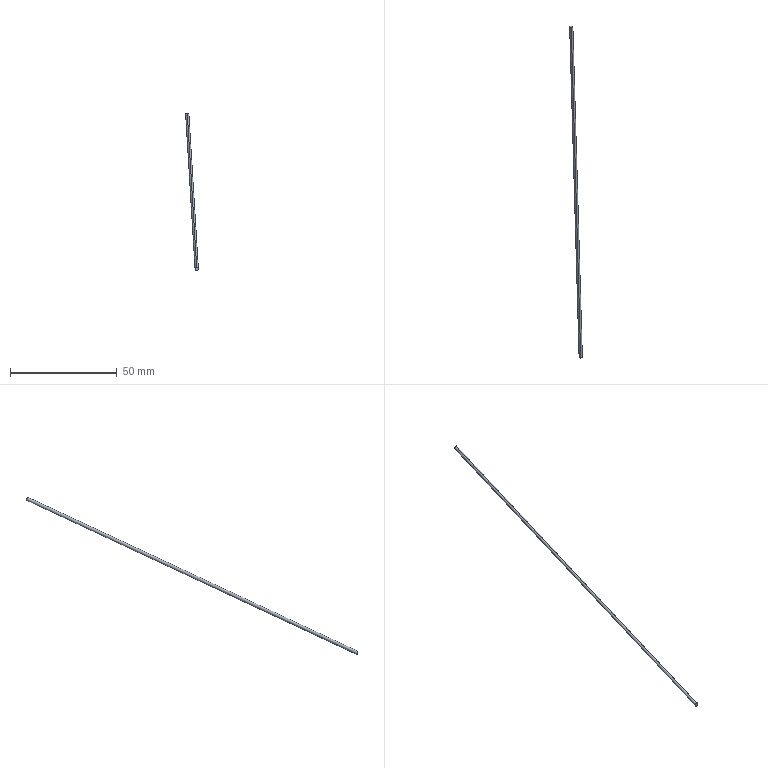Part | STEP file | 1_id790_x_t | 1 solid | 4 faces | box 5.952 x 155.177 x 73.747 mm | volume 311.788 mm3 | cylinder 2 | plane 2 | commonest cylinder face diameters 1.524 x2
STEP:
#1=CARTESIAN_POINT('',(0.,0.,0.));
#2=DIRECTION('',(0.,0.,1.));
#3=DIRECTION('',(1.,0.,0.));
#4=AXIS2_PLACEMENT_3D('',#1,#2,#3);
#5=CARTESIAN_POINT('',(978.112,154.36,-69.251));
#6=VERTEX_POINT('',#5);
#7=CARTESIAN_POINT('',(973.675,309.536,3.114));
#8=VERTEX_POINT('',#7);
#9=CARTESIAN_POINT('',(978.112,154.36,-69.251));
#10=DIRECTION('',(-0.02591,0.906,0.4225));
#11=VECTOR('',#10,1.);
#12=LINE('',#9,#11);
#13=CARTESIAN_POINT('',(976.35,215.719,-39.796));
#14=DIRECTION('',(-0.02591,0.906,0.4225));
#15=DIRECTION('',(0.002266,-0.4226,0.9063));
#16=AXIS2_PLACEMENT_3D('',#13,#14,#15);
#17=CYLINDRICAL_SURFACE('',#16,0.762);
#18=CARTESIAN_POINT('',(3.142,-68.081));
#19=DIRECTION('',(0.,1.));
#20=VECTOR('',#19,1.);
#21=LINE('',#18,#20);
#22=(GEOMETRIC_REPRESENTATION_CONTEXT(2)PARAMETRIC_REPRESENTATION_CONTEXT()REPRESENTATION_CONTEXT('',''));
#23=DEFINITIONAL_REPRESENTATION('',(#21),#22);
#24=PCURVE('',#17,#23);
#25=CARTESIAN_POINT('',(976.35,215.719,-39.796));
#26=DIRECTION('',(-0.02591,0.906,0.4225));
#27=DIRECTION('',(0.002266,-0.4226,0.9063));
#28=AXIS2_PLACEMENT_3D('',#25,#26,#27);
#29=CYLINDRICAL_SURFACE('',#28,0.762);
#30=CARTESIAN_POINT('',(3.142,-68.081));
#31=DIRECTION('',(0.,1.));
#32=VECTOR('',#31,1.);
#33=LINE('',#30,#32);
#34=(GEOMETRIC_REPRESENTATION_CONTEXT(2)PARAMETRIC_REPRESENTATION_CONTEXT()REPRESENTATION_CONTEXT('',''));
#35=DEFINITIONAL_REPRESENTATION('',(#33),#34);
#36=PCURVE('',#29,#35);
#37=SURFACE_CURVE('',#12,(#24,#36),.PCURVE_S1.);
#38=EDGE_CURVE('',#6,#8,#37,.T.);
#39=ORIENTED_EDGE('',*,*,#38,.F.);
#40=CARTESIAN_POINT('',(978.097,154.36,-67.57));
#41=VERTEX_POINT('',#40);
#42=CARTESIAN_POINT('',(978.104,154.36,-68.41));
#43=DIRECTION('',(0.,-1.,0.));
#44=DIRECTION('',(-0.0612,0.,0.9981));
#45=AXIS2_PLACEMENT_3D('',#42,#43,#44);
#46=ELLIPSE('',#45,0.8411,0.762);
#47=CARTESIAN_POINT('',(6.283,-67.37));
#48=CARTESIAN_POINT('',(6.236,-67.369));
#49=CARTESIAN_POINT('',(6.14,-67.37));
#50=CARTESIAN_POINT('',(5.998,-67.378));
#51=CARTESIAN_POINT('',(5.855,-67.393));
#52=CARTESIAN_POINT('',(5.712,-67.414));
#53=CARTESIAN_POINT('',(5.569,-67.443));
#54=CARTESIAN_POINT('',(5.426,-67.476));
#55=CARTESIAN_POINT('',(5.284,-67.515));
#56=CARTESIAN_POINT('',(5.141,-67.559));
#57=CARTESIAN_POINT('',(4.998,-67.605));
#58=CARTESIAN_POINT('',(4.855,-67.654));
#59=CARTESIAN_POINT('',(4.712,-67.705));
#60=CARTESIAN_POINT('',(4.57,-67.756));
#61=CARTESIAN_POINT('',(4.427,-67.806));
#62=CARTESIAN_POINT('',(4.284,-67.855));
#63=CARTESIAN_POINT('',(4.141,-67.901));
#64=CARTESIAN_POINT('',(3.998,-67.944));
#65=CARTESIAN_POINT('',(3.856,-67.982));
#66=CARTESIAN_POINT('',(3.713,-68.014));
#67=CARTESIAN_POINT('',(3.57,-68.041));
#68=CARTESIAN_POINT('',(3.427,-68.062));
#69=CARTESIAN_POINT('',(3.284,-68.076));
#70=CARTESIAN_POINT('',(3.189,-68.08));
#71=CARTESIAN_POINT('',(3.142,-68.081));
#72=B_SPLINE_CURVE_WITH_KNOTS('',3,(#47,#48,#49,#50,#51,#52,#53,#54,#55,#56,#57,#58,#59,#60,#61,#62,#63,#64,#65,#66,#67,#68,#69,#70,#71),.UNSPECIFIED.,.F.,.F.,(4,1,1,1,1,1,1,1,1,1,1,1,1,1,1,1,1,1,1,1,1,1,4),(6.225,6.368,6.511,6.654,6.797,6.939,7.082,7.225,7.368,7.511,7.653,7.796,7.939,8.082,8.225,8.367,8.51,8.653,8.796,8.939,9.081,9.224,9.367),.QUASI_UNIFORM_KNOTS.);
#73=(GEOMETRIC_REPRESENTATION_CONTEXT(2)PARAMETRIC_REPRESENTATION_CONTEXT()REPRESENTATION_CONTEXT('',''));
#74=DEFINITIONAL_REPRESENTATION('',(#72),#73);
#75=PCURVE('',#17,#74);
#76=CARTESIAN_POINT('',(982.853,154.36,-54.26));
#77=DIRECTION('',(0.,-1.,0.));
#78=DIRECTION('',(0.,0.,1.));
#79=AXIS2_PLACEMENT_3D('',#76,#77,#78);
#80=PLANE('',#79);
#81=CARTESIAN_POINT('',(-14.151,4.749));
#82=DIRECTION('',(0.9981,0.0612));
#83=AXIS2_PLACEMENT_2D('',#81,#82);
#84=ELLIPSE('',#83,0.8411,0.762);
#85=(GEOMETRIC_REPRESENTATION_CONTEXT(2)PARAMETRIC_REPRESENTATION_CONTEXT()REPRESENTATION_CONTEXT('',''));
#86=DEFINITIONAL_REPRESENTATION('',(#84),#85);
#87=PCURVE('',#80,#86);
#88=SURFACE_CURVE('',#46,(#75,#87),.PCURVE_S1.);
#89=EDGE_CURVE('',#41,#6,#88,.T.);
#90=ORIENTED_EDGE('',*,*,#89,.F.);
#91=CARTESIAN_POINT('',(973.678,308.892,4.495));
#92=VERTEX_POINT('',#91);
#93=CARTESIAN_POINT('',(978.097,154.36,-67.57));
#94=DIRECTION('',(0.02591,-0.906,-0.4225));
#95=VECTOR('',#94,1.);
#96=LINE('',#93,#95);
#97=CARTESIAN_POINT('',(6.283,-67.37));
#98=DIRECTION('',(0.,-1.));
#99=VECTOR('',#98,1.);
#100=LINE('',#97,#99);
#101=(GEOMETRIC_REPRESENTATION_CONTEXT(2)PARAMETRIC_REPRESENTATION_CONTEXT()REPRESENTATION_CONTEXT('',''));
#102=DEFINITIONAL_REPRESENTATION('',(#100),#101);
#103=PCURVE('',#17,#102);
#104=CARTESIAN_POINT('',(0.,-67.37));
#105=DIRECTION('',(0.,-1.));
#106=VECTOR('',#105,1.);
#107=LINE('',#104,#106);
#108=(GEOMETRIC_REPRESENTATION_CONTEXT(2)PARAMETRIC_REPRESENTATION_CONTEXT()REPRESENTATION_CONTEXT('',''));
#109=DEFINITIONAL_REPRESENTATION('',(#107),#108);
#110=PCURVE('',#29,#109);
#111=SURFACE_CURVE('',#96,(#103,#110),.PCURVE_S1.);
#112=EDGE_CURVE('',#92,#41,#111,.T.);
#113=ORIENTED_EDGE('',*,*,#112,.F.);
#114=CARTESIAN_POINT('',(973.677,309.214,3.805));
#115=DIRECTION('',(-0.02591,0.906,0.4225));
#116=DIRECTION('',(-0.002266,0.4226,-0.9063));
#117=AXIS2_PLACEMENT_3D('',#114,#115,#116);
#118=CIRCLE('',#117,0.762);
#119=CARTESIAN_POINT('',(3.142,103.197));
#120=DIRECTION('',(1.,0.));
#121=VECTOR('',#120,1.);
#122=LINE('',#119,#121);
#123=(GEOMETRIC_REPRESENTATION_CONTEXT(2)PARAMETRIC_REPRESENTATION_CONTEXT()REPRESENTATION_CONTEXT('',''));
#124=DEFINITIONAL_REPRESENTATION('',(#122),#123);
#125=PCURVE('',#17,#124);
#126=CARTESIAN_POINT('',(973.677,309.214,3.805));
#127=DIRECTION('',(0.02591,-0.906,-0.4225));
#128=DIRECTION('',(0.05454,-0.4207,0.9055));
#129=AXIS2_PLACEMENT_3D('',#126,#127,#128);
#130=PLANE('',#129);
#131=CARTESIAN_POINT('',(-0.761,-0.03985));
#132=CARTESIAN_POINT('',(-0.83,1.278));
#133=CARTESIAN_POINT('',(0.346,0.6789));
#134=CARTESIAN_POINT('',(1.522,0.0797));
#135=CARTESIAN_POINT('',(0.415,-0.6391));
#136=CARTESIAN_POINT('',(-0.6919,-1.358));
#137=CARTESIAN_POINT('',(-0.761,-0.03985));
#138=(BOUNDED_CURVE()B_SPLINE_CURVE(2,(#131,#132,#133,#134,#135,#136,#137),.UNSPECIFIED.,.T.,.F.)B_SPLINE_CURVE_WITH_KNOTS((1,2,2,2,2,1),(-2.094,0.,2.094,4.189,6.283,8.378),.UNSPECIFIED.)CURVE()GEOMETRIC_REPRESENTATION_ITEM()RATIONAL_B_SPLINE_CURVE((1.,0.5,1.,0.5,1.,0.5,1.))REPRESENTATION_ITEM(''));
#139=(GEOMETRIC_REPRESENTATION_CONTEXT(2)PARAMETRIC_REPRESENTATION_CONTEXT()REPRESENTATION_CONTEXT('',''));
#140=DEFINITIONAL_REPRESENTATION('',(#138),#139);
#141=PCURVE('',#130,#140);
#142=SURFACE_CURVE('',#118,(#125,#141),.PCURVE_S1.);
#143=EDGE_CURVE('',#8,#92,#142,.T.);
#144=ORIENTED_EDGE('',*,*,#143,.F.);
#145=EDGE_LOOP('',(#39,#90,#113,#144));
#146=FACE_BOUND('',#145,.T.);
#147=ADVANCED_FACE('',(#146),#17,.T.);
#148=ORIENTED_EDGE('',*,*,#143,.T.);
#149=CARTESIAN_POINT('',(973.677,309.214,3.805));
#150=DIRECTION('',(-0.02591,0.906,0.4225));
#151=DIRECTION('',(0.002266,-0.4226,0.9063));
#152=AXIS2_PLACEMENT_3D('',#149,#150,#151);
#153=CIRCLE('',#152,0.762);
#154=CARTESIAN_POINT('',(0.761,0.03985));
#155=CARTESIAN_POINT('',(0.83,-1.278));
#156=CARTESIAN_POINT('',(-0.346,-0.6789));
#157=CARTESIAN_POINT('',(-1.522,-0.0797));
#158=CARTESIAN_POINT('',(-0.415,0.6391));
#159=CARTESIAN_POINT('',(0.6919,1.358));
#160=CARTESIAN_POINT('',(0.761,0.03985));
#161=(BOUNDED_CURVE()B_SPLINE_CURVE(2,(#154,#155,#156,#157,#158,#159,#160),.UNSPECIFIED.,.T.,.F.)B_SPLINE_CURVE_WITH_KNOTS((1,2,2,2,2,1),(-2.094,0.,2.094,4.189,6.283,8.378),.UNSPECIFIED.)CURVE()GEOMETRIC_REPRESENTATION_ITEM()RATIONAL_B_SPLINE_CURVE((1.,0.5,1.,0.5,1.,0.5,1.))REPRESENTATION_ITEM(''));
#162=(GEOMETRIC_REPRESENTATION_CONTEXT(2)PARAMETRIC_REPRESENTATION_CONTEXT()REPRESENTATION_CONTEXT('',''));
#163=DEFINITIONAL_REPRESENTATION('',(#161),#162);
#164=PCURVE('',#130,#163);
#165=CARTESIAN_POINT('',(0.,103.197));
#166=DIRECTION('',(1.,0.));
#167=VECTOR('',#166,1.);
#168=LINE('',#165,#167);
#169=(GEOMETRIC_REPRESENTATION_CONTEXT(2)PARAMETRIC_REPRESENTATION_CONTEXT()REPRESENTATION_CONTEXT('',''));
#170=DEFINITIONAL_REPRESENTATION('',(#168),#169);
#171=PCURVE('',#29,#170);
#172=SURFACE_CURVE('',#153,(#164,#171),.PCURVE_S1.);
#173=EDGE_CURVE('',#92,#8,#172,.T.);
#174=ORIENTED_EDGE('',*,*,#173,.T.);
#175=EDGE_LOOP('',(#148,#174));
#176=FACE_BOUND('',#175,.T.);
#177=ADVANCED_FACE('',(#176),#130,.F.);
#178=ORIENTED_EDGE('',*,*,#112,.T.);
#179=CARTESIAN_POINT('',(978.104,154.36,-68.41));
#180=DIRECTION('',(0.,-1.,0.));
#181=DIRECTION('',(-0.0612,0.,0.9981));
#182=AXIS2_PLACEMENT_3D('',#179,#180,#181);
#183=ELLIPSE('',#182,0.8411,0.762);
#184=CARTESIAN_POINT('',(3.142,-68.081));
#185=CARTESIAN_POINT('',(3.094,-68.082));
#186=CARTESIAN_POINT('',(2.999,-68.082));
#187=CARTESIAN_POINT('',(2.856,-68.074));
#188=CARTESIAN_POINT('',(2.713,-68.059));
#189=CARTESIAN_POINT('',(2.57,-68.037));
#190=CARTESIAN_POINT('',(2.428,-68.009));
#191=CARTESIAN_POINT('',(2.285,-67.975));
#192=CARTESIAN_POINT('',(2.142,-67.936));
#193=CARTESIAN_POINT('',(1.999,-67.892));
#194=CARTESIAN_POINT('',(1.856,-67.846));
#195=CARTESIAN_POINT('',(1.714,-67.797));
#196=CARTESIAN_POINT('',(1.571,-67.746));
#197=CARTESIAN_POINT('',(1.428,-67.695));
#198=CARTESIAN_POINT('',(1.285,-67.645));
#199=CARTESIAN_POINT('',(1.142,-67.596));
#200=CARTESIAN_POINT('',(0.9996,-67.55));
#201=CARTESIAN_POINT('',(0.8568,-67.508));
#202=CARTESIAN_POINT('',(0.714,-67.47));
#203=CARTESIAN_POINT('',(0.5712,-67.437));
#204=CARTESIAN_POINT('',(0.4284,-67.41));
#205=CARTESIAN_POINT('',(0.2856,-67.389));
#206=CARTESIAN_POINT('',(0.1428,-67.376));
#207=CARTESIAN_POINT('',(0.0476,-67.371));
#208=CARTESIAN_POINT('',(0.,-67.37));
#209=B_SPLINE_CURVE_WITH_KNOTS('',3,(#184,#185,#186,#187,#188,#189,#190,#191,#192,#193,#194,#195,#196,#197,#198,#199,#200,#201,#202,#203,#204,#205,#206,#207,#208),.UNSPECIFIED.,.F.,.F.,(4,1,1,1,1,1,1,1,1,1,1,1,1,1,1,1,1,1,1,1,1,1,4),(3.084,3.227,3.369,3.512,3.655,3.798,3.941,4.083,4.226,4.369,4.512,4.655,4.797,4.94,5.083,5.226,5.369,5.511,5.654,5.797,5.94,6.083,6.225),.QUASI_UNIFORM_KNOTS.);
#210=(GEOMETRIC_REPRESENTATION_CONTEXT(2)PARAMETRIC_REPRESENTATION_CONTEXT()REPRESENTATION_CONTEXT('',''));
#211=DEFINITIONAL_REPRESENTATION('',(#209),#210);
#212=PCURVE('',#29,#211);
#213=CARTESIAN_POINT('',(-14.151,4.749));
#214=DIRECTION('',(0.9981,0.0612));
#215=AXIS2_PLACEMENT_2D('',#213,#214);
#216=ELLIPSE('',#215,0.8411,0.762);
#217=(GEOMETRIC_REPRESENTATION_CONTEXT(2)PARAMETRIC_REPRESENTATION_CONTEXT()REPRESENTATION_CONTEXT('',''));
#218=DEFINITIONAL_REPRESENTATION('',(#216),#217);
#219=PCURVE('',#80,#218);
#220=SURFACE_CURVE('',#183,(#212,#219),.PCURVE_S1.);
#221=EDGE_CURVE('',#6,#41,#220,.T.);
#222=ORIENTED_EDGE('',*,*,#221,.F.);
#223=ORIENTED_EDGE('',*,*,#38,.T.);
#224=ORIENTED_EDGE('',*,*,#173,.F.);
#225=EDGE_LOOP('',(#178,#222,#223,#224));
#226=FACE_BOUND('',#225,.T.);
#227=ADVANCED_FACE('',(#226),#29,.T.);
#228=ORIENTED_EDGE('',*,*,#221,.T.);
#229=ORIENTED_EDGE('',*,*,#89,.T.);
#230=EDGE_LOOP('',(#228,#229));
#231=FACE_BOUND('',#230,.T.);
#232=ADVANCED_FACE('',(#231),#80,.T.);
#233=CLOSED_SHELL('',(#147,#177,#227,#232));
#234=MANIFOLD_SOLID_BREP('',#233);
#235=(LENGTH_UNIT()NAMED_UNIT(*)SI_UNIT(.MILLI.,.METRE.));
#236=UNCERTAINTY_MEASURE_WITH_UNIT(LENGTH_MEASURE(0.0000001),#235,'','');
#237=(NAMED_UNIT(*)PLANE_ANGLE_UNIT()SI_UNIT($,.RADIAN.));
#238=(NAMED_UNIT(*)SI_UNIT($,.STERADIAN.)SOLID_ANGLE_UNIT());
#239=(GEOMETRIC_REPRESENTATION_CONTEXT(3)GLOBAL_UNCERTAINTY_ASSIGNED_CONTEXT((#236))GLOBAL_UNIT_ASSIGNED_CONTEXT((#235,#237,#238))REPRESENTATION_CONTEXT('',''));
#240=ADVANCED_BREP_SHAPE_REPRESENTATION('',(#4,#234),#239);